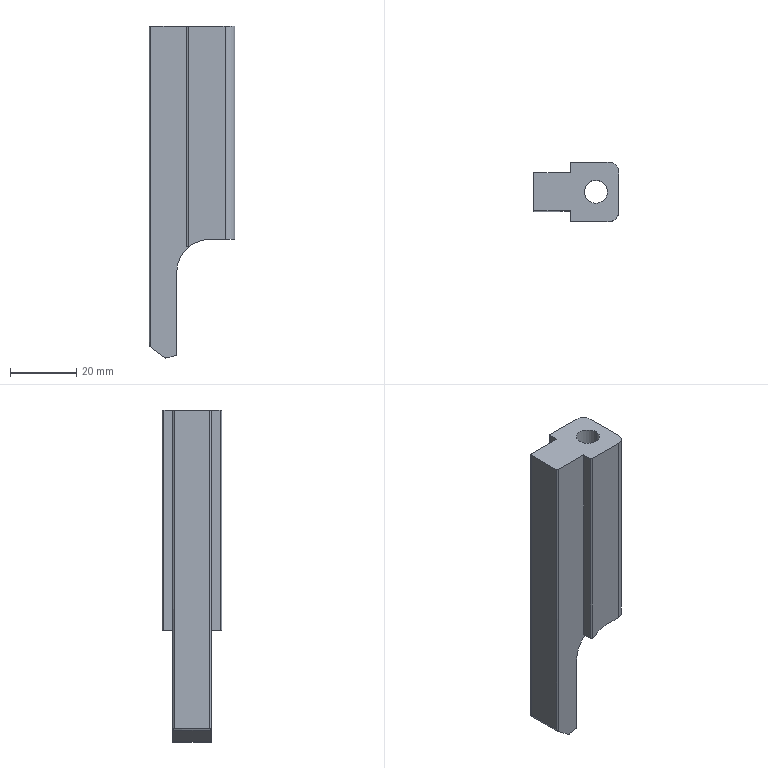Part | 1 solid | 31 faces | box 26 x 18 x 100.48 mm | volume 25656 mm3 | plane 16 | cylinder 15 | commonest cylinder face diameters 1 x6 6 x2 7 x2 11 x2 2 x1 2.074 x1